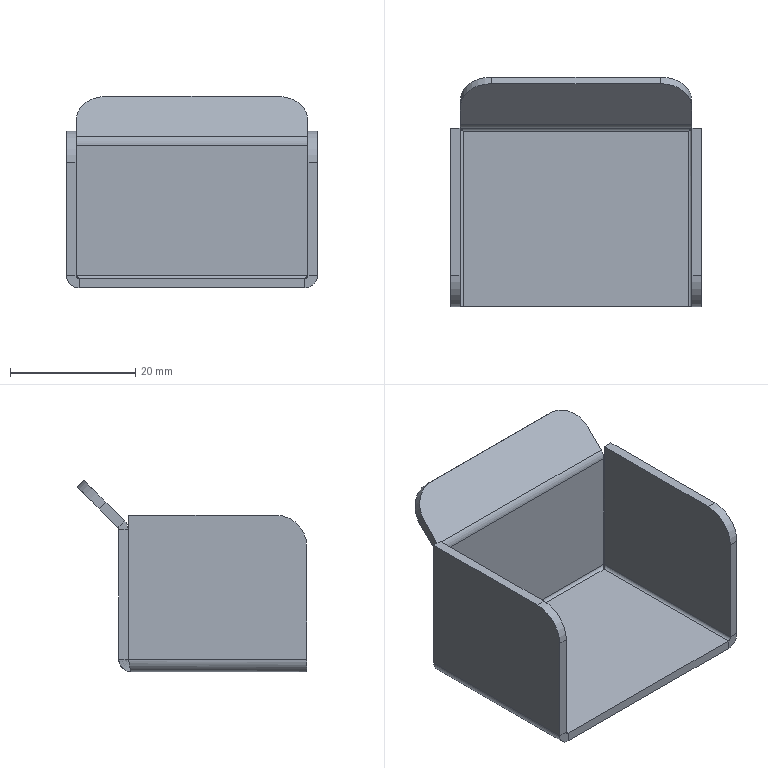Part | SolidWorks | features BaseBody 1 | 1 solid | 42 faces | box 40 x 36.632 x 30.571 mm | volume 5419 mm3 | plane 26 | cylinder 12 | spline 4 | commonest cylinder face diameters 1 x4 4 x4 10 x4
STEP:
#1=CARTESIAN_POINT('',(-13.429,20.571,29.071));
#2=VERTEX_POINT('',#1);
#3=CARTESIAN_POINT('',(-18.429,17.036,25.536));
#4=VERTEX_POINT('',#3);
#5=CARTESIAN_POINT('',(-13.429,17.036,25.536));
#6=DIRECTION('',(0.,-0.7071,0.7071));
#7=DIRECTION('',(0.,0.7071,0.7071));
#8=AXIS2_PLACEMENT_3D('',#5,#6,#7);
#9=CIRCLE('',#8,5.);
#10=EDGE_CURVE('',#2,#4,#9,.T.);
#11=ORIENTED_EDGE('',*,*,#10,.F.);
#12=CARTESIAN_POINT('',(-13.429,21.632,28.01));
#13=VERTEX_POINT('',#12);
#14=CARTESIAN_POINT('',(-13.429,20.571,29.071));
#15=DIRECTION('',(0.,-0.7071,0.7071));
#16=VECTOR('',#15,1000.);
#17=LINE('',#14,#16);
#18=EDGE_CURVE('',#13,#2,#17,.T.);
#19=ORIENTED_EDGE('',*,*,#18,.F.);
#20=CARTESIAN_POINT('',(-18.429,18.096,24.475));
#21=VERTEX_POINT('',#20);
#22=CARTESIAN_POINT('',(-13.429,18.096,24.475));
#23=DIRECTION('',(0.,0.7071,-0.7071));
#24=DIRECTION('',(0.,0.7071,0.7071));
#25=AXIS2_PLACEMENT_3D('',#22,#23,#24);
#26=CIRCLE('',#25,5.);
#27=EDGE_CURVE('',#21,#13,#26,.T.);
#28=ORIENTED_EDGE('',*,*,#27,.F.);
#29=CARTESIAN_POINT('',(-18.429,17.036,25.536));
#30=DIRECTION('',(0.,0.7071,-0.7071));
#31=VECTOR('',#30,1000.);
#32=LINE('',#29,#31);
#33=EDGE_CURVE('',#4,#21,#32,.T.);
#34=ORIENTED_EDGE('',*,*,#33,.F.);
#35=EDGE_LOOP('',(#11,#19,#28,#34));
#36=FACE_OUTER_BOUND('',#35,.T.);
#37=CARTESIAN_POINT('',(-13.429,17.036,25.536));
#38=DIRECTION('',(0.,0.7071,-0.7071));
#39=DIRECTION('',(0.,0.7071,0.7071));
#40=AXIS2_PLACEMENT_3D('',#37,#38,#39);
#41=CYLINDRICAL_SURFACE('',#40,5.);
#42=ADVANCED_FACE('',(#36),#41,.T.);
#43=CARTESIAN_POINT('',(18.429,17.036,25.536));
#44=VERTEX_POINT('',#43);
#45=CARTESIAN_POINT('',(13.429,20.571,29.071));
#46=VERTEX_POINT('',#45);
#47=CARTESIAN_POINT('',(13.429,17.036,25.536));
#48=DIRECTION('',(0.,-0.7071,0.7071));
#49=DIRECTION('',(0.,0.7071,0.7071));
#50=AXIS2_PLACEMENT_3D('',#47,#48,#49);
#51=CIRCLE('',#50,5.);
#52=EDGE_CURVE('',#44,#46,#51,.T.);
#53=ORIENTED_EDGE('',*,*,#52,.F.);
#54=CARTESIAN_POINT('',(18.429,18.096,24.475));
#55=VERTEX_POINT('',#54);
#56=CARTESIAN_POINT('',(18.429,17.036,25.536));
#57=DIRECTION('',(0.,-0.7071,0.7071));
#58=VECTOR('',#57,1000.);
#59=LINE('',#56,#58);
#60=EDGE_CURVE('',#55,#44,#59,.T.);
#61=ORIENTED_EDGE('',*,*,#60,.F.);
#62=CARTESIAN_POINT('',(13.429,21.632,28.01));
#63=VERTEX_POINT('',#62);
#64=CARTESIAN_POINT('',(13.429,18.096,24.475));
#65=DIRECTION('',(0.,0.7071,-0.7071));
#66=DIRECTION('',(0.,0.7071,0.7071));
#67=AXIS2_PLACEMENT_3D('',#64,#65,#66);
#68=CIRCLE('',#67,5.);
#69=EDGE_CURVE('',#63,#55,#68,.T.);
#70=ORIENTED_EDGE('',*,*,#69,.F.);
#71=CARTESIAN_POINT('',(13.429,20.571,29.071));
#72=DIRECTION('',(0.,0.7071,-0.7071));
#73=VECTOR('',#72,1000.);
#74=LINE('',#71,#73);
#75=EDGE_CURVE('',#46,#63,#74,.T.);
#76=ORIENTED_EDGE('',*,*,#75,.F.);
#77=EDGE_LOOP('',(#53,#61,#70,#76));
#78=FACE_OUTER_BOUND('',#77,.T.);
#79=CARTESIAN_POINT('',(13.429,17.036,25.536));
#80=DIRECTION('',(0.,0.7071,-0.7071));
#81=DIRECTION('',(0.,0.7071,0.7071));
#82=AXIS2_PLACEMENT_3D('',#79,#80,#81);
#83=CYLINDRICAL_SURFACE('',#82,5.);
#84=ADVANCED_FACE('',(#78),#83,.T.);
#85=CARTESIAN_POINT('',(20.,-10.,23.5));
#86=VERTEX_POINT('',#85);
#87=CARTESIAN_POINT('',(20.,-15.,18.5));
#88=VERTEX_POINT('',#87);
#89=CARTESIAN_POINT('',(20.,-10.,18.5));
#90=DIRECTION('',(1.,0.,0.));
#91=DIRECTION('',(0.,0.,1.));
#92=AXIS2_PLACEMENT_3D('',#89,#90,#91);
#93=CIRCLE('',#92,5.);
#94=EDGE_CURVE('',#86,#88,#93,.T.);
#95=ORIENTED_EDGE('',*,*,#94,.F.);
#96=CARTESIAN_POINT('',(18.5,-10.,23.5));
#97=VERTEX_POINT('',#96);
#98=CARTESIAN_POINT('',(20.,-10.,23.5));
#99=DIRECTION('',(1.,0.,0.));
#100=VECTOR('',#99,1000.);
#101=LINE('',#98,#100);
#102=EDGE_CURVE('',#97,#86,#101,.T.);
#103=ORIENTED_EDGE('',*,*,#102,.F.);
#104=CARTESIAN_POINT('',(18.5,-15.,18.5));
#105=VERTEX_POINT('',#104);
#106=CARTESIAN_POINT('',(18.5,-10.,18.5));
#107=DIRECTION('',(-1.,0.,0.));
#108=DIRECTION('',(0.,0.,1.));
#109=AXIS2_PLACEMENT_3D('',#106,#107,#108);
#110=CIRCLE('',#109,5.);
#111=EDGE_CURVE('',#105,#97,#110,.T.);
#112=ORIENTED_EDGE('',*,*,#111,.F.);
#113=CARTESIAN_POINT('',(20.,-15.,18.5));
#114=DIRECTION('',(-1.,0.,0.));
#115=VECTOR('',#114,1000.);
#116=LINE('',#113,#115);
#117=EDGE_CURVE('',#88,#105,#116,.T.);
#118=ORIENTED_EDGE('',*,*,#117,.F.);
#119=EDGE_LOOP('',(#95,#103,#112,#118));
#120=FACE_OUTER_BOUND('',#119,.T.);
#121=CARTESIAN_POINT('',(20.,-10.,18.5));
#122=DIRECTION('',(-1.,0.,0.));
#123=DIRECTION('',(0.,0.,1.));
#124=AXIS2_PLACEMENT_3D('',#121,#122,#123);
#125=CYLINDRICAL_SURFACE('',#124,5.);
#126=ADVANCED_FACE('',(#120),#125,.T.);
#127=CARTESIAN_POINT('',(-20.,-15.,18.5));
#128=VERTEX_POINT('',#127);
#129=CARTESIAN_POINT('',(-20.,-10.,23.5));
#130=VERTEX_POINT('',#129);
#131=CARTESIAN_POINT('',(-20.,-10.,18.5));
#132=DIRECTION('',(-1.,0.,0.));
#133=DIRECTION('',(0.,0.,-1.));
#134=AXIS2_PLACEMENT_3D('',#131,#132,#133);
#135=CIRCLE('',#134,5.);
#136=EDGE_CURVE('',#128,#130,#135,.T.);
#137=ORIENTED_EDGE('',*,*,#136,.F.);
#138=CARTESIAN_POINT('',(-18.5,-15.,18.5));
#139=VERTEX_POINT('',#138);
#140=CARTESIAN_POINT('',(-20.,-15.,18.5));
#141=DIRECTION('',(-1.,0.,0.));
#142=VECTOR('',#141,1000.);
#143=LINE('',#140,#142);
#144=EDGE_CURVE('',#139,#128,#143,.T.);
#145=ORIENTED_EDGE('',*,*,#144,.F.);
#146=CARTESIAN_POINT('',(-18.5,-10.,23.5));
#147=VERTEX_POINT('',#146);
#148=CARTESIAN_POINT('',(-18.5,-10.,18.5));
#149=DIRECTION('',(1.,0.,0.));
#150=DIRECTION('',(0.,0.,-1.));
#151=AXIS2_PLACEMENT_3D('',#148,#149,#150);
#152=CIRCLE('',#151,5.);
#153=EDGE_CURVE('',#147,#139,#152,.T.);
#154=ORIENTED_EDGE('',*,*,#153,.F.);
#155=CARTESIAN_POINT('',(-20.,-10.,23.5));
#156=DIRECTION('',(1.,0.,0.));
#157=VECTOR('',#156,1000.);
#158=LINE('',#155,#157);
#159=EDGE_CURVE('',#130,#147,#158,.T.);
#160=ORIENTED_EDGE('',*,*,#159,.F.);
#161=EDGE_LOOP('',(#137,#145,#154,#160));
#162=FACE_OUTER_BOUND('',#161,.T.);
#163=CARTESIAN_POINT('',(-20.,-10.,18.5));
#164=DIRECTION('',(1.,0.,0.));
#165=DIRECTION('',(0.,0.,-1.));
#166=AXIS2_PLACEMENT_3D('',#163,#164,#165);
#167=CYLINDRICAL_SURFACE('',#166,5.);
#168=ADVANCED_FACE('',(#162),#167,.T.);
#169=CARTESIAN_POINT('',(0.,20.571,29.071));
#170=DIRECTION('',(-1.,0.,0.));
#171=VECTOR('',#170,1000.);
#172=LINE('',#169,#171);
#173=EDGE_CURVE('',#46,#2,#172,.T.);
#174=ORIENTED_EDGE('',*,*,#173,.F.);
#175=ORIENTED_EDGE('',*,*,#75,.T.);
#176=CARTESIAN_POINT('',(-18.429,21.632,28.01));
#177=DIRECTION('',(-1.,0.,0.));
#178=VECTOR('',#177,1000.);
#179=LINE('',#176,#178);
#180=EDGE_CURVE('',#63,#13,#179,.T.);
#181=ORIENTED_EDGE('',*,*,#180,.T.);
#182=ORIENTED_EDGE('',*,*,#18,.T.);
#183=EDGE_LOOP('',(#174,#175,#181,#182));
#184=FACE_OUTER_BOUND('',#183,.T.);
#185=CARTESIAN_POINT('',(-18.429,20.571,29.071));
#186=DIRECTION('',(0.,-0.7071,-0.7071));
#187=DIRECTION('',(0.,-0.7071,0.7071));
#188=AXIS2_PLACEMENT_3D('',#185,#186,#187);
#189=PLANE('',#188);
#190=ADVANCED_FACE('',(#184),#189,.F.);
#191=ORIENTED_EDGE('',*,*,#180,.F.);
#192=ORIENTED_EDGE('',*,*,#69,.T.);
#193=CARTESIAN_POINT('',(18.429,15.146,21.525));
#194=VERTEX_POINT('',#193);
#195=CARTESIAN_POINT('',(18.429,21.632,28.01));
#196=DIRECTION('',(0.,0.7071,0.7071));
#197=VECTOR('',#196,1000.);
#198=LINE('',#195,#197);
#199=EDGE_CURVE('',#194,#55,#198,.T.);
#200=ORIENTED_EDGE('',*,*,#199,.F.);
#201=CARTESIAN_POINT('',(-18.429,15.146,21.525));
#202=VERTEX_POINT('',#201);
#203=CARTESIAN_POINT('',(-18.429,15.146,21.525));
#204=DIRECTION('',(1.,0.,0.));
#205=VECTOR('',#204,1000.);
#206=LINE('',#203,#205);
#207=EDGE_CURVE('',#202,#194,#206,.T.);
#208=ORIENTED_EDGE('',*,*,#207,.F.);
#209=CARTESIAN_POINT('',(-18.429,15.,21.379));
#210=DIRECTION('',(0.,-0.7071,-0.7071));
#211=VECTOR('',#210,1000.);
#212=LINE('',#209,#211);
#213=EDGE_CURVE('',#21,#202,#212,.T.);
#214=ORIENTED_EDGE('',*,*,#213,.F.);
#215=ORIENTED_EDGE('',*,*,#27,.T.);
#216=EDGE_LOOP('',(#191,#192,#200,#208,#214,#215));
#217=FACE_OUTER_BOUND('',#216,.T.);
#218=CARTESIAN_POINT('',(0.,-4.25,2.129));
#219=DIRECTION('',(0.,0.7071,-0.7071));
#220=DIRECTION('',(-1.,0.,0.));
#221=AXIS2_PLACEMENT_3D('',#218,#219,#220);
#222=PLANE('',#221);
#223=ADVANCED_FACE('',(#217),#222,.T.);
#224=CARTESIAN_POINT('',(18.429,14.086,22.586));
#225=VERTEX_POINT('',#224);
#226=CARTESIAN_POINT('',(18.429,-5.311,3.189));
#227=DIRECTION('',(0.,0.7071,0.7071));
#228=VECTOR('',#227,1000.);
#229=LINE('',#226,#228);
#230=EDGE_CURVE('',#225,#44,#229,.T.);
#231=ORIENTED_EDGE('',*,*,#230,.T.);
#232=ORIENTED_EDGE('',*,*,#52,.T.);
#233=ORIENTED_EDGE('',*,*,#173,.T.);
#234=ORIENTED_EDGE('',*,*,#10,.T.);
#235=CARTESIAN_POINT('',(-18.429,14.086,22.586));
#236=VERTEX_POINT('',#235);
#237=CARTESIAN_POINT('',(-18.429,-5.311,3.189));
#238=DIRECTION('',(0.,-0.7071,-0.7071));
#239=VECTOR('',#238,1000.);
#240=LINE('',#237,#239);
#241=EDGE_CURVE('',#4,#236,#240,.T.);
#242=ORIENTED_EDGE('',*,*,#241,.T.);
#243=CARTESIAN_POINT('',(-18.429,14.086,22.586));
#244=DIRECTION('',(-1.,0.,0.));
#245=VECTOR('',#244,1000.);
#246=LINE('',#243,#245);
#247=EDGE_CURVE('',#225,#236,#246,.T.);
#248=ORIENTED_EDGE('',*,*,#247,.F.);
#249=EDGE_LOOP('',(#231,#232,#233,#234,#242,#248));
#250=FACE_OUTER_BOUND('',#249,.T.);
#251=CARTESIAN_POINT('',(0.,-5.311,3.189));
#252=DIRECTION('',(0.,0.7071,-0.7071));
#253=DIRECTION('',(-1.,0.,0.));
#254=AXIS2_PLACEMENT_3D('',#251,#252,#253);
#255=PLANE('',#254);
#256=ADVANCED_FACE('',(#250),#255,.F.);
#257=ORIENTED_EDGE('',*,*,#199,.T.);
#258=ORIENTED_EDGE('',*,*,#60,.T.);
#259=ORIENTED_EDGE('',*,*,#230,.F.);
#260=CARTESIAN_POINT('',(18.429,15.146,21.525));
#261=DIRECTION('',(0.,-0.7071,0.7071));
#262=VECTOR('',#261,1000.);
#263=LINE('',#260,#262);
#264=EDGE_CURVE('',#194,#225,#263,.T.);
#265=ORIENTED_EDGE('',*,*,#264,.F.);
#266=EDGE_LOOP('',(#257,#258,#259,#265));
#267=FACE_OUTER_BOUND('',#266,.T.);
#268=CARTESIAN_POINT('',(18.429,20.571,29.071));
#269=DIRECTION('',(-1.,0.,0.));
#270=DIRECTION('',(0.,1.,0.));
#271=AXIS2_PLACEMENT_3D('',#268,#269,#270);
#272=PLANE('',#271);
#273=ADVANCED_FACE('',(#267),#272,.F.);
#274=ORIENTED_EDGE('',*,*,#241,.F.);
#275=ORIENTED_EDGE('',*,*,#33,.T.);
#276=ORIENTED_EDGE('',*,*,#213,.T.);
#277=CARTESIAN_POINT('',(-18.429,14.086,22.586));
#278=DIRECTION('',(0.,-0.7071,0.7071));
#279=VECTOR('',#278,1000.);
#280=LINE('',#277,#279);
#281=EDGE_CURVE('',#202,#236,#280,.T.);
#282=ORIENTED_EDGE('',*,*,#281,.T.);
#283=EDGE_LOOP('',(#274,#275,#276,#282));
#284=FACE_OUTER_BOUND('',#283,.T.);
#285=CARTESIAN_POINT('',(-18.429,13.939,22.439));
#286=DIRECTION('',(1.,0.,0.));
#287=DIRECTION('',(0.,1.,0.));
#288=AXIS2_PLACEMENT_3D('',#285,#286,#287);
#289=PLANE('',#288);
#290=ADVANCED_FACE('',(#284),#289,.F.);
#291=CARTESIAN_POINT('',(18.429,15.,21.172));
#292=VERTEX_POINT('',#291);
#293=CARTESIAN_POINT('',(-18.429,15.,21.172));
#294=VERTEX_POINT('',#293);
#295=CARTESIAN_POINT('',(18.429,15.,21.172));
#296=DIRECTION('',(-1.,0.,0.));
#297=VECTOR('',#296,1000.);
#298=LINE('',#295,#297);
#299=EDGE_CURVE('',#292,#294,#298,.T.);
#300=ORIENTED_EDGE('',*,*,#299,.T.);
#301=CARTESIAN_POINT('',(-18.429,15.5,21.172));
#302=DIRECTION('',(-1.,0.,0.));
#303=DIRECTION('',(0.,0.,-1.));
#304=AXIS2_PLACEMENT_3D('',#301,#302,#303);
#305=CIRCLE('',#304,0.5);
#306=EDGE_CURVE('',#294,#202,#305,.T.);
#307=ORIENTED_EDGE('',*,*,#306,.T.);
#308=ORIENTED_EDGE('',*,*,#207,.T.);
#309=CARTESIAN_POINT('',(18.429,15.5,21.172));
#310=DIRECTION('',(1.,0.,0.));
#311=DIRECTION('',(0.,0.,-1.));
#312=AXIS2_PLACEMENT_3D('',#309,#310,#311);
#313=CIRCLE('',#312,0.5);
#314=EDGE_CURVE('',#194,#292,#313,.T.);
#315=ORIENTED_EDGE('',*,*,#314,.T.);
#316=EDGE_LOOP('',(#300,#307,#308,#315));
#317=FACE_OUTER_BOUND('',#316,.T.);
#318=CARTESIAN_POINT('',(18.429,15.5,21.172));
#319=DIRECTION('',(1.,0.,0.));
#320=DIRECTION('',(0.,-0.7071,0.7071));
#321=AXIS2_PLACEMENT_3D('',#318,#319,#320);
#322=CYLINDRICAL_SURFACE('',#321,0.5);
#323=ADVANCED_FACE('',(#317),#322,.F.);
#324=CARTESIAN_POINT('',(18.429,13.5,21.172));
#325=VERTEX_POINT('',#324);
#326=CARTESIAN_POINT('',(-18.429,13.5,21.172));
#327=VERTEX_POINT('',#326);
#328=CARTESIAN_POINT('',(18.429,13.5,21.172));
#329=DIRECTION('',(-1.,0.,0.));
#330=VECTOR('',#329,1000.);
#331=LINE('',#328,#330);
#332=EDGE_CURVE('',#325,#327,#331,.T.);
#333=ORIENTED_EDGE('',*,*,#332,.F.);
#334=CARTESIAN_POINT('',(18.429,15.5,21.172));
#335=DIRECTION('',(1.,0.,0.));
#336=DIRECTION('',(0.,0.,-1.));
#337=AXIS2_PLACEMENT_3D('',#334,#335,#336);
#338=CIRCLE('',#337,2.);
#339=EDGE_CURVE('',#225,#325,#338,.T.);
#340=ORIENTED_EDGE('',*,*,#339,.F.);
#341=ORIENTED_EDGE('',*,*,#247,.T.);
#342=CARTESIAN_POINT('',(-18.429,15.5,21.172));
#343=DIRECTION('',(-1.,0.,0.));
#344=DIRECTION('',(0.,0.,-1.));
#345=AXIS2_PLACEMENT_3D('',#342,#343,#344);
#346=CIRCLE('',#345,2.);
#347=EDGE_CURVE('',#327,#236,#346,.T.);
#348=ORIENTED_EDGE('',*,*,#347,.F.);
#349=EDGE_LOOP('',(#333,#340,#341,#348));
#350=FACE_OUTER_BOUND('',#349,.T.);
#351=CARTESIAN_POINT('',(18.429,15.5,21.172));
#352=DIRECTION('',(1.,0.,0.));
#353=DIRECTION('',(0.,-0.7071,0.7071));
#354=AXIS2_PLACEMENT_3D('',#351,#352,#353);
#355=CYLINDRICAL_SURFACE('',#354,2.);
#356=ADVANCED_FACE('',(#350),#355,.T.);
#357=ORIENTED_EDGE('',*,*,#314,.F.);
#358=ORIENTED_EDGE('',*,*,#264,.T.);
#359=ORIENTED_EDGE('',*,*,#339,.T.);
#360=CARTESIAN_POINT('',(18.429,15.,21.172));
#361=DIRECTION('',(0.,-1.,0.));
#362=VECTOR('',#361,1000.);
#363=LINE('',#360,#362);
#364=EDGE_CURVE('',#292,#325,#363,.T.);
#365=ORIENTED_EDGE('',*,*,#364,.F.);
#366=EDGE_LOOP('',(#357,#358,#359,#365));
#367=FACE_OUTER_BOUND('',#366,.T.);
#368=CARTESIAN_POINT('',(18.429,15.5,21.172));
#369=DIRECTION('',(-1.,0.,0.));
#370=DIRECTION('',(0.,0.,1.));
#371=AXIS2_PLACEMENT_3D('',#368,#369,#370);
#372=PLANE('',#371);
#373=ADVANCED_FACE('',(#367),#372,.F.);
#374=ORIENTED_EDGE('',*,*,#281,.F.);
#375=ORIENTED_EDGE('',*,*,#306,.F.);
#376=CARTESIAN_POINT('',(-18.429,15.,21.172));
#377=DIRECTION('',(0.,-1.,0.));
#378=VECTOR('',#377,1000.);
#379=LINE('',#376,#378);
#380=EDGE_CURVE('',#294,#327,#379,.T.);
#381=ORIENTED_EDGE('',*,*,#380,.T.);
#382=ORIENTED_EDGE('',*,*,#347,.T.);
#383=EDGE_LOOP('',(#374,#375,#381,#382));
#384=FACE_OUTER_BOUND('',#383,.T.);
#385=CARTESIAN_POINT('',(-18.429,15.5,21.172));
#386=DIRECTION('',(-1.,0.,0.));
#387=DIRECTION('',(0.,0.,1.));
#388=AXIS2_PLACEMENT_3D('',#385,#386,#387);
#389=PLANE('',#388);
#390=ADVANCED_FACE('',(#384),#389,.T.);
#391=CARTESIAN_POINT('',(20.,13.429,23.5));
#392=VERTEX_POINT('',#391);
#393=CARTESIAN_POINT('',(18.5,13.429,23.5));
#394=VERTEX_POINT('',#393);
#395=CARTESIAN_POINT('',(20.,13.429,23.5));
#396=DIRECTION('',(-1.,0.,0.));
#397=VECTOR('',#396,1000.);
#398=LINE('',#395,#397);
#399=EDGE_CURVE('',#392,#394,#398,.T.);
#400=ORIENTED_EDGE('',*,*,#399,.F.);
#401=CARTESIAN_POINT('',(20.,13.429,0.5));
#402=VERTEX_POINT('',#401);
#403=CARTESIAN_POINT('',(20.,13.429,0.));
#404=DIRECTION('',(0.,0.,1.));
#405=VECTOR('',#404,1000.);
#406=LINE('',#403,#405);
#407=EDGE_CURVE('',#402,#392,#406,.T.);
#408=ORIENTED_EDGE('',*,*,#407,.F.);
#409=CARTESIAN_POINT('',(18.5,13.429,0.5));
#410=VERTEX_POINT('',#409);
#411=CARTESIAN_POINT('',(18.5,13.429,0.5));
#412=DIRECTION('',(-1.,0.,0.));
#413=VECTOR('',#412,1000.);
#414=LINE('',#411,#413);
#415=EDGE_CURVE('',#402,#410,#414,.T.);
#416=ORIENTED_EDGE('',*,*,#415,.T.);
#417=CARTESIAN_POINT('',(18.5,13.429,0.));
#418=DIRECTION('',(0.,0.,1.));
#419=VECTOR('',#418,1000.);
#420=LINE('',#417,#419);
#421=EDGE_CURVE('',#410,#394,#420,.T.);
#422=ORIENTED_EDGE('',*,*,#421,.T.);
#423=EDGE_LOOP('',(#400,#408,#416,#422));
#424=FACE_OUTER_BOUND('',#423,.T.);
#425=CARTESIAN_POINT('',(18.5,13.429,0.));
#426=DIRECTION('',(0.,-1.,0.));
#427=DIRECTION('',(0.,0.,-1.));
#428=AXIS2_PLACEMENT_3D('',#425,#426,#427);
#429=PLANE('',#428);
#430=ADVANCED_FACE('',(#424),#429,.F.);
#431=CARTESIAN_POINT('',(18.5,-15.,23.5));
#432=DIRECTION('',(0.,-1.,0.));
#433=VECTOR('',#432,1000.);
#434=LINE('',#431,#433);
#435=EDGE_CURVE('',#394,#97,#434,.T.);
#436=ORIENTED_EDGE('',*,*,#435,.T.);
#437=ORIENTED_EDGE('',*,*,#102,.T.);
#438=CARTESIAN_POINT('',(20.,0.,23.5));
#439=DIRECTION('',(0.,-1.,0.));
#440=VECTOR('',#439,1000.);
#441=LINE('',#438,#440);
#442=EDGE_CURVE('',#392,#86,#441,.T.);
#443=ORIENTED_EDGE('',*,*,#442,.F.);
#444=ORIENTED_EDGE('',*,*,#399,.T.);
#445=EDGE_LOOP('',(#436,#437,#443,#444));
#446=FACE_OUTER_BOUND('',#445,.T.);
#447=CARTESIAN_POINT('',(20.,-15.,23.5));
#448=DIRECTION('',(0.,0.,-1.));
#449=DIRECTION('',(-1.,0.,0.));
#450=AXIS2_PLACEMENT_3D('',#447,#448,#449);
#451=PLANE('',#450);
#452=ADVANCED_FACE('',(#446),#451,.F.);
#453=CARTESIAN_POINT('',(18.5,-15.,0.5));
#454=VERTEX_POINT('',#453);
#455=CARTESIAN_POINT('',(18.5,-15.,0.));
#456=DIRECTION('',(0.,0.,-1.));
#457=VECTOR('',#456,1000.);
#458=LINE('',#455,#457);
#459=EDGE_CURVE('',#105,#454,#458,.T.);
#460=ORIENTED_EDGE('',*,*,#459,.F.);
#461=ORIENTED_EDGE('',*,*,#111,.T.);
#462=ORIENTED_EDGE('',*,*,#435,.F.);
#463=ORIENTED_EDGE('',*,*,#421,.F.);
#464=CARTESIAN_POINT('',(18.5,-15.,0.5));
#465=DIRECTION('',(0.,1.,0.));
#466=VECTOR('',#465,1000.);
#467=LINE('',#464,#466);
#468=EDGE_CURVE('',#454,#410,#467,.T.);
#469=ORIENTED_EDGE('',*,*,#468,.F.);
#470=EDGE_LOOP('',(#460,#461,#462,#463,#469));
#471=FACE_OUTER_BOUND('',#470,.T.);
#472=CARTESIAN_POINT('',(18.5,0.,0.));
#473=DIRECTION('',(-1.,0.,0.));
#474=DIRECTION('',(0.,1.,0.));
#475=AXIS2_PLACEMENT_3D('',#472,#473,#474);
#476=PLANE('',#475);
#477=ADVANCED_FACE('',(#471),#476,.T.);
#478=ORIENTED_EDGE('',*,*,#442,.T.);
#479=ORIENTED_EDGE('',*,*,#94,.T.);
#480=CARTESIAN_POINT('',(20.,-15.,0.5));
#481=VERTEX_POINT('',#480);
#482=CARTESIAN_POINT('',(20.,-15.,0.));
#483=DIRECTION('',(0.,0.,-1.));
#484=VECTOR('',#483,1000.);
#485=LINE('',#482,#484);
#486=EDGE_CURVE('',#88,#481,#485,.T.);
#487=ORIENTED_EDGE('',*,*,#486,.T.);
#488=CARTESIAN_POINT('',(20.,-15.,0.5));
#489=DIRECTION('',(0.,-1.,0.));
#490=VECTOR('',#489,1000.);
#491=LINE('',#488,#490);
#492=EDGE_CURVE('',#402,#481,#491,.T.);
#493=ORIENTED_EDGE('',*,*,#492,.F.);
#494=ORIENTED_EDGE('',*,*,#407,.T.);
#495=EDGE_LOOP('',(#478,#479,#487,#493,#494));
#496=FACE_OUTER_BOUND('',#495,.T.);
#497=CARTESIAN_POINT('',(20.,0.,0.));
#498=DIRECTION('',(-1.,0.,0.));
#499=DIRECTION('',(0.,1.,0.));
#500=AXIS2_PLACEMENT_3D('',#497,#498,#499);
#501=PLANE('',#500);
#502=ADVANCED_FACE('',(#496),#501,.F.);
#503=ORIENTED_EDGE('',*,*,#486,.F.);
#504=ORIENTED_EDGE('',*,*,#117,.T.);
#505=ORIENTED_EDGE('',*,*,#459,.T.);
#506=CARTESIAN_POINT('',(20.,-15.,0.5));
#507=DIRECTION('',(1.,0.,0.));
#508=VECTOR('',#507,1000.);
#509=LINE('',#506,#508);
#510=EDGE_CURVE('',#454,#481,#509,.T.);
#511=ORIENTED_EDGE('',*,*,#510,.T.);
#512=EDGE_LOOP('',(#503,#504,#505,#511));
#513=FACE_OUTER_BOUND('',#512,.T.);
#514=CARTESIAN_POINT('',(20.,-15.,0.));
#515=DIRECTION('',(0.,1.,0.));
#516=DIRECTION('',(0.,0.,-1.));
#517=AXIS2_PLACEMENT_3D('',#514,#515,#516);
#518=PLANE('',#517);
#519=ADVANCED_FACE('',(#513),#518,.F.);
#520=CARTESIAN_POINT('',(18.,13.,0.));
#521=VERTEX_POINT('',#520);
#522=CARTESIAN_POINT('',(18.,-15.,0.));
#523=VERTEX_POINT('',#522);
#524=CARTESIAN_POINT('',(18.,13.429,0.));
#525=DIRECTION('',(0.,-1.,0.));
#526=VECTOR('',#525,1000.);
#527=LINE('',#524,#526);
#528=EDGE_CURVE('',#521,#523,#527,.T.);
#529=ORIENTED_EDGE('',*,*,#528,.T.);
#530=CARTESIAN_POINT('',(18.,-15.,0.5));
#531=DIRECTION('',(0.,-1.,0.));
#532=DIRECTION('',(0.,0.,1.));
#533=AXIS2_PLACEMENT_3D('',#530,#531,#532);
#534=CIRCLE('',#533,0.5);
#535=EDGE_CURVE('',#523,#454,#534,.T.);
#536=ORIENTED_EDGE('',*,*,#535,.T.);
#537=ORIENTED_EDGE('',*,*,#468,.T.);
#538=CARTESIAN_POINT('',(18.5,13.429,0.5));
#539=CARTESIAN_POINT('',(18.5,13.358,0.3691));
#540=CARTESIAN_POINT('',(18.446,13.286,0.239));
#541=CARTESIAN_POINT('',(18.261,13.143,0.05389));
#542=CARTESIAN_POINT('',(18.131,13.072,0.));
#543=CARTESIAN_POINT('',(18.,13.,0.));
#544=B_SPLINE_CURVE_WITH_KNOTS('',3,(#538,#539,#540,#541,#542,#543),.UNSPECIFIED.,.F.,.F.,(4,2,4),(0.,0.5,1.),.UNSPECIFIED.);
#545=EDGE_CURVE('',#410,#521,#544,.T.);
#546=ORIENTED_EDGE('',*,*,#545,.T.);
#547=EDGE_LOOP('',(#529,#536,#537,#546));
#548=FACE_OUTER_BOUND('',#547,.T.);
#549=CARTESIAN_POINT('',(18.,13.429,0.5));
#550=DIRECTION('',(0.,1.,0.));
#551=DIRECTION('',(1.,0.,0.));
#552=AXIS2_PLACEMENT_3D('',#549,#550,#551);
#553=CYLINDRICAL_SURFACE('',#552,0.5);
#554=ADVANCED_FACE('',(#548),#553,.F.);
#555=CARTESIAN_POINT('',(18.,13.,-1.5));
#556=VERTEX_POINT('',#555);
#557=CARTESIAN_POINT('',(18.,-15.,-1.5));
#558=VERTEX_POINT('',#557);
#559=CARTESIAN_POINT('',(18.,13.429,-1.5));
#560=DIRECTION('',(0.,-1.,0.));
#561=VECTOR('',#560,1000.);
#562=LINE('',#559,#561);
#563=EDGE_CURVE('',#556,#558,#562,.T.);
#564=ORIENTED_EDGE('',*,*,#563,.F.);
#565=CARTESIAN_POINT('',(20.,13.429,0.5));
#566=CARTESIAN_POINT('',(20.,13.394,0.2382));
#567=CARTESIAN_POINT('',(19.948,13.358,-0.0235));
#568=CARTESIAN_POINT('',(19.748,13.286,-0.5072));
#569=CARTESIAN_POINT('',(19.599,13.25,-0.7291));
#570=CARTESIAN_POINT('',(19.229,13.179,-1.099));
#571=CARTESIAN_POINT('',(19.007,13.143,-1.248));
#572=CARTESIAN_POINT('',(18.523,13.072,-1.448));
#573=CARTESIAN_POINT('',(18.262,13.036,-1.5));
#574=CARTESIAN_POINT('',(18.,13.,-1.5));
#575=B_SPLINE_CURVE_WITH_KNOTS('',3,(#565,#566,#567,#568,#569,#570,#571,#572,#573,#574),.UNSPECIFIED.,.F.,.F.,(4,2,2,2,4),(0.,0.25,0.5,0.75,1.),.UNSPECIFIED.);
#576=EDGE_CURVE('',#402,#556,#575,.T.);
#577=ORIENTED_EDGE('',*,*,#576,.F.);
#578=ORIENTED_EDGE('',*,*,#492,.T.);
#579=CARTESIAN_POINT('',(18.,-15.,0.5));
#580=DIRECTION('',(0.,-1.,0.));
#581=DIRECTION('',(0.,0.,1.));
#582=AXIS2_PLACEMENT_3D('',#579,#580,#581);
#583=CIRCLE('',#582,2.);
#584=EDGE_CURVE('',#558,#481,#583,.T.);
#585=ORIENTED_EDGE('',*,*,#584,.F.);
#586=EDGE_LOOP('',(#564,#577,#578,#585));
#587=FACE_OUTER_BOUND('',#586,.T.);
#588=CARTESIAN_POINT('',(18.,13.429,0.5));
#589=DIRECTION('',(0.,1.,0.));
#590=DIRECTION('',(1.,0.,0.));
#591=AXIS2_PLACEMENT_3D('',#588,#589,#590);
#592=CYLINDRICAL_SURFACE('',#591,2.);
#593=ADVANCED_FACE('',(#587),#592,.T.);
#594=ORIENTED_EDGE('',*,*,#545,.F.);
#595=ORIENTED_EDGE('',*,*,#415,.F.);
#596=ORIENTED_EDGE('',*,*,#576,.T.);
#597=CARTESIAN_POINT('',(18.,13.,0.));
#598=DIRECTION('',(0.,0.,-1.));
#599=VECTOR('',#598,1000.);
#600=LINE('',#597,#599);
#601=EDGE_CURVE('',#521,#556,#600,.T.);
#602=ORIENTED_EDGE('',*,*,#601,.F.);
#603=EDGE_LOOP('',(#594,#595,#596,#602));
#604=FACE_OUTER_BOUND('',#603,.T.);
#605=CARTESIAN_POINT('',(20.015,13.429,0.5));
#606=CARTESIAN_POINT('',(20.015,13.394,0.2362));
#607=CARTESIAN_POINT('',(19.963,13.358,-0.02742));
#608=CARTESIAN_POINT('',(19.761,13.286,-0.5148));
#609=CARTESIAN_POINT('',(19.611,13.25,-0.7383));
#610=CARTESIAN_POINT('',(19.238,13.179,-1.111));
#611=CARTESIAN_POINT('',(19.015,13.143,-1.261));
#612=CARTESIAN_POINT('',(18.527,13.072,-1.463));
#613=CARTESIAN_POINT('',(18.264,13.036,-1.515));
#614=CARTESIAN_POINT('',(18.,13.,-1.515));
#615=CARTESIAN_POINT('',(20.,13.429,0.5));
#616=CARTESIAN_POINT('',(20.,13.394,0.2382));
#617=CARTESIAN_POINT('',(19.948,13.358,-0.0235));
#618=CARTESIAN_POINT('',(19.748,13.286,-0.5072));
#619=CARTESIAN_POINT('',(19.599,13.25,-0.7291));
#620=CARTESIAN_POINT('',(19.229,13.179,-1.099));
#621=CARTESIAN_POINT('',(19.007,13.143,-1.248));
#622=CARTESIAN_POINT('',(18.523,13.072,-1.448));
#623=CARTESIAN_POINT('',(18.262,13.036,-1.5));
#624=CARTESIAN_POINT('',(18.,13.,-1.5));
#625=CARTESIAN_POINT('',(18.5,13.429,0.5));
#626=CARTESIAN_POINT('',(18.5,13.394,0.4345));
#627=CARTESIAN_POINT('',(18.487,13.358,0.3691));
#628=CARTESIAN_POINT('',(18.437,13.286,0.2482));
#629=CARTESIAN_POINT('',(18.4,13.25,0.1927));
#630=CARTESIAN_POINT('',(18.307,13.179,0.1002));
#631=CARTESIAN_POINT('',(18.252,13.143,0.06311));
#632=CARTESIAN_POINT('',(18.131,13.072,0.01301));
#633=CARTESIAN_POINT('',(18.065,13.036,0.));
#634=CARTESIAN_POINT('',(18.,13.,0.));
#635=CARTESIAN_POINT('',(18.485,13.429,0.5));
#636=CARTESIAN_POINT('',(18.485,13.394,0.4365));
#637=CARTESIAN_POINT('',(18.472,13.358,0.3731));
#638=CARTESIAN_POINT('',(18.424,13.286,0.2558));
#639=CARTESIAN_POINT('',(18.388,13.25,0.202));
#640=CARTESIAN_POINT('',(18.298,13.179,0.1123));
#641=CARTESIAN_POINT('',(18.244,13.143,0.07634));
#642=CARTESIAN_POINT('',(18.127,13.072,0.02777));
#643=CARTESIAN_POINT('',(18.063,13.036,0.01515));
#644=CARTESIAN_POINT('',(18.,13.,0.01515));
#645=B_SPLINE_SURFACE_WITH_KNOTS('',1,3,((#605,#606,#607,#608,#609,#610,#611,#612,#613,#614),(#615,#616,#617,#618,#619,#620,#621,#622,#623,#624),(#625,#626,#627,#628,#629,#630,#631,#632,#633,#634),(#635,#636,#637,#638,#639,#640,#641,#642,#643,#644)),.UNSPECIFIED.,.F.,.F.,.F.,(2,1,1,2),(4,2,2,2,4),(-0.01,0.,1.,1.01),(0.,0.25,0.5,0.75,1.),.UNSPECIFIED.);
#646=ADVANCED_FACE('',(#604),#645,.F.);
#647=ORIENTED_EDGE('',*,*,#510,.F.);
#648=ORIENTED_EDGE('',*,*,#535,.F.);
#649=CARTESIAN_POINT('',(18.,-15.,0.));
#650=DIRECTION('',(0.,0.,-1.));
#651=VECTOR('',#650,1000.);
#652=LINE('',#649,#651);
#653=EDGE_CURVE('',#523,#558,#652,.T.);
#654=ORIENTED_EDGE('',*,*,#653,.T.);
#655=ORIENTED_EDGE('',*,*,#584,.T.);
#656=EDGE_LOOP('',(#647,#648,#654,#655));
#657=FACE_OUTER_BOUND('',#656,.T.);
#658=CARTESIAN_POINT('',(18.,-15.,0.5));
#659=DIRECTION('',(0.,-1.,0.));
#660=DIRECTION('',(-1.,0.,0.));
#661=AXIS2_PLACEMENT_3D('',#658,#659,#660);
#662=PLANE('',#661);
#663=ADVANCED_FACE('',(#657),#662,.T.);
#664=CARTESIAN_POINT('',(-18.,13.,0.));
#665=VERTEX_POINT('',#664);
#666=CARTESIAN_POINT('',(-18.429,13.,0.));
#667=DIRECTION('',(1.,0.,0.));
#668=VECTOR('',#667,1000.);
#669=LINE('',#666,#668);
#670=EDGE_CURVE('',#665,#521,#669,.T.);
#671=ORIENTED_EDGE('',*,*,#670,.T.);
#672=CARTESIAN_POINT('',(18.429,13.5,0.5));
#673=VERTEX_POINT('',#672);
#674=CARTESIAN_POINT('',(18.,13.,0.));
#675=CARTESIAN_POINT('',(18.072,13.131,0.));
#676=CARTESIAN_POINT('',(18.143,13.261,0.05389));
#677=CARTESIAN_POINT('',(18.286,13.446,0.239));
#678=CARTESIAN_POINT('',(18.358,13.5,0.3691));
#679=CARTESIAN_POINT('',(18.429,13.5,0.5));
#680=B_SPLINE_CURVE_WITH_KNOTS('',3,(#674,#675,#676,#677,#678,#679),.UNSPECIFIED.,.F.,.F.,(4,2,4),(0.,0.5,1.),.UNSPECIFIED.);
#681=EDGE_CURVE('',#521,#673,#680,.T.);
#682=ORIENTED_EDGE('',*,*,#681,.T.);
#683=CARTESIAN_POINT('',(-18.429,13.5,0.5));
#684=VERTEX_POINT('',#683);
#685=CARTESIAN_POINT('',(20.,13.5,0.5));
#686=DIRECTION('',(-1.,0.,0.));
#687=VECTOR('',#686,1000.);
#688=LINE('',#685,#687);
#689=EDGE_CURVE('',#673,#684,#688,.T.);
#690=ORIENTED_EDGE('',*,*,#689,.T.);
#691=CARTESIAN_POINT('',(-18.429,13.5,0.5));
#692=CARTESIAN_POINT('',(-18.358,13.5,0.3691));
#693=CARTESIAN_POINT('',(-18.286,13.446,0.239));
#694=CARTESIAN_POINT('',(-18.143,13.261,0.05389));
#695=CARTESIAN_POINT('',(-18.072,13.131,0.));
#696=CARTESIAN_POINT('',(-18.,13.,0.));
#697=B_SPLINE_CURVE_WITH_KNOTS('',3,(#691,#692,#693,#694,#695,#696),.UNSPECIFIED.,.F.,.F.,(4,2,4),(0.,0.5,1.),.UNSPECIFIED.);
#698=EDGE_CURVE('',#684,#665,#697,.T.);
#699=ORIENTED_EDGE('',*,*,#698,.T.);
#700=EDGE_LOOP('',(#671,#682,#690,#699));
#701=FACE_OUTER_BOUND('',#700,.T.);
#702=CARTESIAN_POINT('',(-18.429,13.,0.5));
#703=DIRECTION('',(-1.,0.,0.));
#704=DIRECTION('',(0.,1.,0.));
#705=AXIS2_PLACEMENT_3D('',#702,#703,#704);
#706=CYLINDRICAL_SURFACE('',#705,0.5);
#707=ADVANCED_FACE('',(#701),#706,.F.);
#708=CARTESIAN_POINT('',(-18.,13.,-1.5));
#709=VERTEX_POINT('',#708);
#710=CARTESIAN_POINT('',(-18.429,13.,-1.5));
#711=DIRECTION('',(1.,0.,0.));
#712=VECTOR('',#711,1000.);
#713=LINE('',#710,#712);
#714=EDGE_CURVE('',#709,#556,#713,.T.);
#715=ORIENTED_EDGE('',*,*,#714,.F.);
#716=CARTESIAN_POINT('',(-18.429,15.,0.5));
#717=VERTEX_POINT('',#716);
#718=CARTESIAN_POINT('',(-18.429,15.,0.5));
#719=CARTESIAN_POINT('',(-18.394,15.,0.2382));
#720=CARTESIAN_POINT('',(-18.358,14.948,-0.0235));
#721=CARTESIAN_POINT('',(-18.286,14.748,-0.5072));
#722=CARTESIAN_POINT('',(-18.25,14.599,-0.7291));
#723=CARTESIAN_POINT('',(-18.179,14.229,-1.099));
#724=CARTESIAN_POINT('',(-18.143,14.007,-1.248));
#725=CARTESIAN_POINT('',(-18.072,13.523,-1.448));
#726=CARTESIAN_POINT('',(-18.036,13.262,-1.5));
#727=CARTESIAN_POINT('',(-18.,13.,-1.5));
#728=B_SPLINE_CURVE_WITH_KNOTS('',3,(#718,#719,#720,#721,#722,#723,#724,#725,#726,#727),.UNSPECIFIED.,.F.,.F.,(4,2,2,2,4),(0.,0.25,0.5,0.75,1.),.UNSPECIFIED.);
#729=EDGE_CURVE('',#717,#709,#728,.T.);
#730=ORIENTED_EDGE('',*,*,#729,.F.);
#731=CARTESIAN_POINT('',(18.429,15.,0.5));
#732=VERTEX_POINT('',#731);
#733=CARTESIAN_POINT('',(20.,15.,0.5));
#734=DIRECTION('',(1.,0.,0.));
#735=VECTOR('',#734,1000.);
#736=LINE('',#733,#735);
#737=EDGE_CURVE('',#717,#732,#736,.T.);
#738=ORIENTED_EDGE('',*,*,#737,.T.);
#739=CARTESIAN_POINT('',(18.,13.,-1.5));
#740=CARTESIAN_POINT('',(18.036,13.262,-1.5));
#741=CARTESIAN_POINT('',(18.072,13.523,-1.448));
#742=CARTESIAN_POINT('',(18.143,14.007,-1.248));
#743=CARTESIAN_POINT('',(18.179,14.229,-1.099));
#744=CARTESIAN_POINT('',(18.25,14.599,-0.7291));
#745=CARTESIAN_POINT('',(18.286,14.748,-0.5072));
#746=CARTESIAN_POINT('',(18.358,14.948,-0.0235));
#747=CARTESIAN_POINT('',(18.394,15.,0.2382));
#748=CARTESIAN_POINT('',(18.429,15.,0.5));
#749=B_SPLINE_CURVE_WITH_KNOTS('',3,(#739,#740,#741,#742,#743,#744,#745,#746,#747,#748),.UNSPECIFIED.,.F.,.F.,(4,2,2,2,4),(0.,0.25,0.5,0.75,1.),.UNSPECIFIED.);
#750=EDGE_CURVE('',#556,#732,#749,.T.);
#751=ORIENTED_EDGE('',*,*,#750,.F.);
#752=EDGE_LOOP('',(#715,#730,#738,#751));
#753=FACE_OUTER_BOUND('',#752,.T.);
#754=CARTESIAN_POINT('',(-18.429,13.,0.5));
#755=DIRECTION('',(-1.,0.,0.));
#756=DIRECTION('',(0.,1.,0.));
#757=AXIS2_PLACEMENT_3D('',#754,#755,#756);
#758=CYLINDRICAL_SURFACE('',#757,2.);
#759=ADVANCED_FACE('',(#753),#758,.T.);
#760=ORIENTED_EDGE('',*,*,#698,.F.);
#761=CARTESIAN_POINT('',(-18.429,13.5,0.5));
#762=DIRECTION('',(0.,-1.,0.));
#763=VECTOR('',#762,1000.);
#764=LINE('',#761,#763);
#765=EDGE_CURVE('',#717,#684,#764,.T.);
#766=ORIENTED_EDGE('',*,*,#765,.F.);
#767=ORIENTED_EDGE('',*,*,#729,.T.);
#768=CARTESIAN_POINT('',(-18.,13.,0.));
#769=DIRECTION('',(0.,0.,-1.));
#770=VECTOR('',#769,1000.);
#771=LINE('',#768,#770);
#772=EDGE_CURVE('',#665,#709,#771,.T.);
#773=ORIENTED_EDGE('',*,*,#772,.F.);
#774=EDGE_LOOP('',(#760,#766,#767,#773));
#775=FACE_OUTER_BOUND('',#774,.T.);
#776=CARTESIAN_POINT('',(-18.429,15.015,0.5));
#777=CARTESIAN_POINT('',(-18.394,15.015,0.2362));
#778=CARTESIAN_POINT('',(-18.358,14.963,-0.02742));
#779=CARTESIAN_POINT('',(-18.286,14.761,-0.5148));
#780=CARTESIAN_POINT('',(-18.25,14.611,-0.7383));
#781=CARTESIAN_POINT('',(-18.179,14.238,-1.111));
#782=CARTESIAN_POINT('',(-18.143,14.015,-1.261));
#783=CARTESIAN_POINT('',(-18.072,13.527,-1.463));
#784=CARTESIAN_POINT('',(-18.036,13.264,-1.515));
#785=CARTESIAN_POINT('',(-18.,13.,-1.515));
#786=CARTESIAN_POINT('',(-18.429,15.,0.5));
#787=CARTESIAN_POINT('',(-18.394,15.,0.2382));
#788=CARTESIAN_POINT('',(-18.358,14.948,-0.0235));
#789=CARTESIAN_POINT('',(-18.286,14.748,-0.5072));
#790=CARTESIAN_POINT('',(-18.25,14.599,-0.7291));
#791=CARTESIAN_POINT('',(-18.179,14.229,-1.099));
#792=CARTESIAN_POINT('',(-18.143,14.007,-1.248));
#793=CARTESIAN_POINT('',(-18.072,13.523,-1.448));
#794=CARTESIAN_POINT('',(-18.036,13.262,-1.5));
#795=CARTESIAN_POINT('',(-18.,13.,-1.5));
#796=CARTESIAN_POINT('',(-18.429,13.5,0.5));
#797=CARTESIAN_POINT('',(-18.394,13.5,0.4345));
#798=CARTESIAN_POINT('',(-18.358,13.487,0.3691));
#799=CARTESIAN_POINT('',(-18.286,13.437,0.2482));
#800=CARTESIAN_POINT('',(-18.25,13.4,0.1927));
#801=CARTESIAN_POINT('',(-18.179,13.307,0.1002));
#802=CARTESIAN_POINT('',(-18.143,13.252,0.06311));
#803=CARTESIAN_POINT('',(-18.072,13.131,0.01301));
#804=CARTESIAN_POINT('',(-18.036,13.065,0.));
#805=CARTESIAN_POINT('',(-18.,13.,0.));
#806=CARTESIAN_POINT('',(-18.429,13.485,0.5));
#807=CARTESIAN_POINT('',(-18.394,13.485,0.4365));
#808=CARTESIAN_POINT('',(-18.358,13.472,0.3731));
#809=CARTESIAN_POINT('',(-18.286,13.424,0.2558));
#810=CARTESIAN_POINT('',(-18.25,13.388,0.202));
#811=CARTESIAN_POINT('',(-18.179,13.298,0.1123));
#812=CARTESIAN_POINT('',(-18.143,13.244,0.07634));
#813=CARTESIAN_POINT('',(-18.072,13.127,0.02777));
#814=CARTESIAN_POINT('',(-18.036,13.063,0.01515));
#815=CARTESIAN_POINT('',(-18.,13.,0.01515));
#816=B_SPLINE_SURFACE_WITH_KNOTS('',1,3,((#776,#777,#778,#779,#780,#781,#782,#783,#784,#785),(#786,#787,#788,#789,#790,#791,#792,#793,#794,#795),(#796,#797,#798,#799,#800,#801,#802,#803,#804,#805),(#806,#807,#808,#809,#810,#811,#812,#813,#814,#815)),.UNSPECIFIED.,.F.,.F.,.F.,(2,1,1,2),(4,2,2,2,4),(-0.01,0.,1.,1.01),(0.,0.25,0.5,0.75,1.),.UNSPECIFIED.);
#817=ADVANCED_FACE('',(#775),#816,.F.);
#818=CARTESIAN_POINT('',(18.429,13.5,0.5));
#819=DIRECTION('',(0.,-1.,0.));
#820=VECTOR('',#819,1000.);
#821=LINE('',#818,#820);
#822=EDGE_CURVE('',#732,#673,#821,.T.);
#823=ORIENTED_EDGE('',*,*,#822,.T.);
#824=ORIENTED_EDGE('',*,*,#681,.F.);
#825=ORIENTED_EDGE('',*,*,#601,.T.);
#826=ORIENTED_EDGE('',*,*,#750,.T.);
#827=EDGE_LOOP('',(#823,#824,#825,#826));
#828=FACE_OUTER_BOUND('',#827,.T.);
#829=CARTESIAN_POINT('',(18.,13.,-1.515));
#830=CARTESIAN_POINT('',(18.036,13.264,-1.515));
#831=CARTESIAN_POINT('',(18.072,13.527,-1.463));
#832=CARTESIAN_POINT('',(18.143,14.015,-1.261));
#833=CARTESIAN_POINT('',(18.179,14.238,-1.111));
#834=CARTESIAN_POINT('',(18.25,14.611,-0.7383));
#835=CARTESIAN_POINT('',(18.286,14.761,-0.5148));
#836=CARTESIAN_POINT('',(18.358,14.963,-0.02742));
#837=CARTESIAN_POINT('',(18.394,15.015,0.2362));
#838=CARTESIAN_POINT('',(18.429,15.015,0.5));
#839=CARTESIAN_POINT('',(18.,13.,-1.5));
#840=CARTESIAN_POINT('',(18.036,13.262,-1.5));
#841=CARTESIAN_POINT('',(18.072,13.523,-1.448));
#842=CARTESIAN_POINT('',(18.143,14.007,-1.248));
#843=CARTESIAN_POINT('',(18.179,14.229,-1.099));
#844=CARTESIAN_POINT('',(18.25,14.599,-0.7291));
#845=CARTESIAN_POINT('',(18.286,14.748,-0.5072));
#846=CARTESIAN_POINT('',(18.358,14.948,-0.0235));
#847=CARTESIAN_POINT('',(18.394,15.,0.2382));
#848=CARTESIAN_POINT('',(18.429,15.,0.5));
#849=CARTESIAN_POINT('',(18.,13.,0.));
#850=CARTESIAN_POINT('',(18.036,13.065,0.));
#851=CARTESIAN_POINT('',(18.072,13.131,0.01301));
#852=CARTESIAN_POINT('',(18.143,13.252,0.06311));
#853=CARTESIAN_POINT('',(18.179,13.307,0.1002));
#854=CARTESIAN_POINT('',(18.25,13.4,0.1927));
#855=CARTESIAN_POINT('',(18.286,13.437,0.2482));
#856=CARTESIAN_POINT('',(18.358,13.487,0.3691));
#857=CARTESIAN_POINT('',(18.394,13.5,0.4345));
#858=CARTESIAN_POINT('',(18.429,13.5,0.5));
#859=CARTESIAN_POINT('',(18.,13.,0.01515));
#860=CARTESIAN_POINT('',(18.036,13.063,0.01515));
#861=CARTESIAN_POINT('',(18.072,13.127,0.02777));
#862=CARTESIAN_POINT('',(18.143,13.244,0.07634));
#863=CARTESIAN_POINT('',(18.179,13.298,0.1123));
#864=CARTESIAN_POINT('',(18.25,13.388,0.202));
#865=CARTESIAN_POINT('',(18.286,13.424,0.2558));
#866=CARTESIAN_POINT('',(18.358,13.472,0.3731));
#867=CARTESIAN_POINT('',(18.394,13.485,0.4365));
#868=CARTESIAN_POINT('',(18.429,13.485,0.5));
#869=B_SPLINE_SURFACE_WITH_KNOTS('',1,3,((#829,#830,#831,#832,#833,#834,#835,#836,#837,#838),(#839,#840,#841,#842,#843,#844,#845,#846,#847,#848),(#849,#850,#851,#852,#853,#854,#855,#856,#857,#858),(#859,#860,#861,#862,#863,#864,#865,#866,#867,#868)),.UNSPECIFIED.,.F.,.F.,.F.,(2,1,1,2),(4,2,2,2,4),(-0.01,0.,1.,1.01),(0.,0.25,0.5,0.75,1.),.UNSPECIFIED.);
#870=ADVANCED_FACE('',(#828),#869,.F.);
#871=CARTESIAN_POINT('',(-18.5,-15.,0.5));
#872=VERTEX_POINT('',#871);
#873=CARTESIAN_POINT('',(-18.5,-15.,23.5));
#874=DIRECTION('',(0.,0.,1.));
#875=VECTOR('',#874,1000.);
#876=LINE('',#873,#875);
#877=EDGE_CURVE('',#872,#139,#876,.T.);
#878=ORIENTED_EDGE('',*,*,#877,.T.);
#879=ORIENTED_EDGE('',*,*,#144,.T.);
#880=CARTESIAN_POINT('',(-20.,-15.,0.5));
#881=VERTEX_POINT('',#880);
#882=CARTESIAN_POINT('',(-20.,-15.,0.));
#883=DIRECTION('',(0.,0.,1.));
#884=VECTOR('',#883,1000.);
#885=LINE('',#882,#884);
#886=EDGE_CURVE('',#881,#128,#885,.T.);
#887=ORIENTED_EDGE('',*,*,#886,.F.);
#888=CARTESIAN_POINT('',(-18.5,-15.,0.5));
#889=DIRECTION('',(-1.,0.,0.));
#890=VECTOR('',#889,1000.);
#891=LINE('',#888,#890);
#892=EDGE_CURVE('',#872,#881,#891,.T.);
#893=ORIENTED_EDGE('',*,*,#892,.F.);
#894=EDGE_LOOP('',(#878,#879,#887,#893));
#895=FACE_OUTER_BOUND('',#894,.T.);
#896=CARTESIAN_POINT('',(-20.,-15.,23.5));
#897=DIRECTION('',(0.,1.,0.));
#898=DIRECTION('',(1.,0.,0.));
#899=AXIS2_PLACEMENT_3D('',#896,#897,#898);
#900=PLANE('',#899);
#901=ADVANCED_FACE('',(#895),#900,.F.);
#902=CARTESIAN_POINT('',(-20.,13.429,23.5));
#903=VERTEX_POINT('',#902);
#904=CARTESIAN_POINT('',(-20.,0.,23.5));
#905=DIRECTION('',(0.,1.,0.));
#906=VECTOR('',#905,1000.);
#907=LINE('',#904,#906);
#908=EDGE_CURVE('',#130,#903,#907,.T.);
#909=ORIENTED_EDGE('',*,*,#908,.F.);
#910=ORIENTED_EDGE('',*,*,#159,.T.);
#911=CARTESIAN_POINT('',(-18.5,13.429,23.5));
#912=VERTEX_POINT('',#911);
#913=CARTESIAN_POINT('',(-18.5,15.,23.5));
#914=DIRECTION('',(0.,1.,0.));
#915=VECTOR('',#914,1000.);
#916=LINE('',#913,#915);
#917=EDGE_CURVE('',#147,#912,#916,.T.);
#918=ORIENTED_EDGE('',*,*,#917,.T.);
#919=CARTESIAN_POINT('',(-18.5,13.429,23.5));
#920=DIRECTION('',(1.,0.,0.));
#921=VECTOR('',#920,1000.);
#922=LINE('',#919,#921);
#923=EDGE_CURVE('',#903,#912,#922,.T.);
#924=ORIENTED_EDGE('',*,*,#923,.F.);
#925=EDGE_LOOP('',(#909,#910,#918,#924));
#926=FACE_OUTER_BOUND('',#925,.T.);
#927=CARTESIAN_POINT('',(-20.,15.,23.5));
#928=DIRECTION('',(0.,0.,-1.));
#929=DIRECTION('',(0.,-1.,0.));
#930=AXIS2_PLACEMENT_3D('',#927,#928,#929);
#931=PLANE('',#930);
#932=ADVANCED_FACE('',(#926),#931,.F.);
#933=ORIENTED_EDGE('',*,*,#917,.F.);
#934=ORIENTED_EDGE('',*,*,#153,.T.);
#935=ORIENTED_EDGE('',*,*,#877,.F.);
#936=CARTESIAN_POINT('',(-18.5,13.429,0.5));
#937=VERTEX_POINT('',#936);
#938=CARTESIAN_POINT('',(-18.5,15.,0.5));
#939=DIRECTION('',(0.,-1.,0.));
#940=VECTOR('',#939,1000.);
#941=LINE('',#938,#940);
#942=EDGE_CURVE('',#937,#872,#941,.T.);
#943=ORIENTED_EDGE('',*,*,#942,.F.);
#944=CARTESIAN_POINT('',(-18.5,13.429,0.));
#945=DIRECTION('',(0.,0.,1.));
#946=VECTOR('',#945,1000.);
#947=LINE('',#944,#946);
#948=EDGE_CURVE('',#937,#912,#947,.T.);
#949=ORIENTED_EDGE('',*,*,#948,.T.);
#950=EDGE_LOOP('',(#933,#934,#935,#943,#949));
#951=FACE_OUTER_BOUND('',#950,.T.);
#952=CARTESIAN_POINT('',(-18.5,0.,0.));
#953=DIRECTION('',(1.,0.,0.));
#954=DIRECTION('',(0.,0.,1.));
#955=AXIS2_PLACEMENT_3D('',#952,#953,#954);
#956=PLANE('',#955);
#957=ADVANCED_FACE('',(#951),#956,.T.);
#958=ORIENTED_EDGE('',*,*,#886,.T.);
#959=ORIENTED_EDGE('',*,*,#136,.T.);
#960=ORIENTED_EDGE('',*,*,#908,.T.);
#961=CARTESIAN_POINT('',(-20.,13.429,0.5));
#962=VERTEX_POINT('',#961);
#963=CARTESIAN_POINT('',(-20.,13.429,0.));
#964=DIRECTION('',(0.,0.,1.));
#965=VECTOR('',#964,1000.);
#966=LINE('',#963,#965);
#967=EDGE_CURVE('',#962,#903,#966,.T.);
#968=ORIENTED_EDGE('',*,*,#967,.F.);
#969=CARTESIAN_POINT('',(-20.,15.,0.5));
#970=DIRECTION('',(0.,1.,0.));
#971=VECTOR('',#970,1000.);
#972=LINE('',#969,#971);
#973=EDGE_CURVE('',#881,#962,#972,.T.);
#974=ORIENTED_EDGE('',*,*,#973,.F.);
#975=EDGE_LOOP('',(#958,#959,#960,#968,#974));
#976=FACE_OUTER_BOUND('',#975,.T.);
#977=CARTESIAN_POINT('',(-20.,0.,0.));
#978=DIRECTION('',(1.,0.,0.));
#979=DIRECTION('',(0.,0.,1.));
#980=AXIS2_PLACEMENT_3D('',#977,#978,#979);
#981=PLANE('',#980);
#982=ADVANCED_FACE('',(#976),#981,.F.);
#983=ORIENTED_EDGE('',*,*,#967,.T.);
#984=ORIENTED_EDGE('',*,*,#923,.T.);
#985=ORIENTED_EDGE('',*,*,#948,.F.);
#986=CARTESIAN_POINT('',(-18.5,13.429,0.5));
#987=DIRECTION('',(1.,0.,0.));
#988=VECTOR('',#987,1000.);
#989=LINE('',#986,#988);
#990=EDGE_CURVE('',#962,#937,#989,.T.);
#991=ORIENTED_EDGE('',*,*,#990,.F.);
#992=EDGE_LOOP('',(#983,#984,#985,#991));
#993=FACE_OUTER_BOUND('',#992,.T.);
#994=CARTESIAN_POINT('',(-18.5,13.429,0.));
#995=DIRECTION('',(0.,1.,0.));
#996=DIRECTION('',(1.,0.,0.));
#997=AXIS2_PLACEMENT_3D('',#994,#995,#996);
#998=PLANE('',#997);
#999=ADVANCED_FACE('',(#993),#998,.T.);
#1000=CARTESIAN_POINT('',(-18.,-15.,0.));
#1001=VERTEX_POINT('',#1000);
#1002=CARTESIAN_POINT('',(-18.,-15.,0.));
#1003=DIRECTION('',(0.,1.,0.));
#1004=VECTOR('',#1003,1000.);
#1005=LINE('',#1002,#1004);
#1006=EDGE_CURVE('',#1001,#665,#1005,.T.);
#1007=ORIENTED_EDGE('',*,*,#1006,.T.);
#1008=CARTESIAN_POINT('',(-18.,13.,0.));
#1009=CARTESIAN_POINT('',(-18.131,13.072,0.));
#1010=CARTESIAN_POINT('',(-18.261,13.143,0.05389));
#1011=CARTESIAN_POINT('',(-18.446,13.286,0.239));
#1012=CARTESIAN_POINT('',(-18.5,13.358,0.3691));
#1013=CARTESIAN_POINT('',(-18.5,13.429,0.5));
#1014=B_SPLINE_CURVE_WITH_KNOTS('',3,(#1008,#1009,#1010,#1011,#1012,#1013),.UNSPECIFIED.,.F.,.F.,(4,2,4),(0.,0.5,1.),.UNSPECIFIED.);
#1015=EDGE_CURVE('',#665,#937,#1014,.T.);
#1016=ORIENTED_EDGE('',*,*,#1015,.T.);
#1017=ORIENTED_EDGE('',*,*,#942,.T.);
#1018=CARTESIAN_POINT('',(-18.,-15.,0.5));
#1019=DIRECTION('',(0.,-1.,0.));
#1020=DIRECTION('',(0.,0.,-1.));
#1021=AXIS2_PLACEMENT_3D('',#1018,#1019,#1020);
#1022=CIRCLE('',#1021,0.5);
#1023=EDGE_CURVE('',#872,#1001,#1022,.T.);
#1024=ORIENTED_EDGE('',*,*,#1023,.T.);
#1025=EDGE_LOOP('',(#1007,#1016,#1017,#1024));
#1026=FACE_OUTER_BOUND('',#1025,.T.);
#1027=CARTESIAN_POINT('',(-18.,-15.,0.5));
#1028=DIRECTION('',(0.,-1.,0.));
#1029=DIRECTION('',(-1.,0.,0.));
#1030=AXIS2_PLACEMENT_3D('',#1027,#1028,#1029);
#1031=CYLINDRICAL_SURFACE('',#1030,0.5);
#1032=ADVANCED_FACE('',(#1026),#1031,.F.);
#1033=CARTESIAN_POINT('',(-18.,-15.,-1.5));
#1034=VERTEX_POINT('',#1033);
#1035=CARTESIAN_POINT('',(-18.,-15.,-1.5));
#1036=DIRECTION('',(0.,1.,0.));
#1037=VECTOR('',#1036,1000.);
#1038=LINE('',#1035,#1037);
#1039=EDGE_CURVE('',#1034,#709,#1038,.T.);
#1040=ORIENTED_EDGE('',*,*,#1039,.F.);
#1041=CARTESIAN_POINT('',(-18.,-15.,0.5));
#1042=DIRECTION('',(0.,-1.,0.));
#1043=DIRECTION('',(0.,0.,-1.));
#1044=AXIS2_PLACEMENT_3D('',#1041,#1042,#1043);
#1045=CIRCLE('',#1044,2.);
#1046=EDGE_CURVE('',#881,#1034,#1045,.T.);
#1047=ORIENTED_EDGE('',*,*,#1046,.F.);
#1048=ORIENTED_EDGE('',*,*,#973,.T.);
#1049=CARTESIAN_POINT('',(-18.,13.,-1.5));
#1050=CARTESIAN_POINT('',(-18.262,13.036,-1.5));
#1051=CARTESIAN_POINT('',(-18.523,13.072,-1.448));
#1052=CARTESIAN_POINT('',(-19.007,13.143,-1.248));
#1053=CARTESIAN_POINT('',(-19.229,13.179,-1.099));
#1054=CARTESIAN_POINT('',(-19.599,13.25,-0.7291));
#1055=CARTESIAN_POINT('',(-19.748,13.286,-0.5072));
#1056=CARTESIAN_POINT('',(-19.948,13.358,-0.0235));
#1057=CARTESIAN_POINT('',(-20.,13.394,0.2382));
#1058=CARTESIAN_POINT('',(-20.,13.429,0.5));
#1059=B_SPLINE_CURVE_WITH_KNOTS('',3,(#1049,#1050,#1051,#1052,#1053,#1054,#1055,#1056,#1057,#1058),.UNSPECIFIED.,.F.,.F.,(4,2,2,2,4),(0.,0.25,0.5,0.75,1.),.UNSPECIFIED.);
#1060=EDGE_CURVE('',#709,#962,#1059,.T.);
#1061=ORIENTED_EDGE('',*,*,#1060,.F.);
#1062=EDGE_LOOP('',(#1040,#1047,#1048,#1061));
#1063=FACE_OUTER_BOUND('',#1062,.T.);
#1064=CARTESIAN_POINT('',(-18.,-15.,0.5));
#1065=DIRECTION('',(0.,-1.,0.));
#1066=DIRECTION('',(-1.,0.,0.));
#1067=AXIS2_PLACEMENT_3D('',#1064,#1065,#1066);
#1068=CYLINDRICAL_SURFACE('',#1067,2.);
#1069=ADVANCED_FACE('',(#1063),#1068,.T.);
#1070=ORIENTED_EDGE('',*,*,#1023,.F.);
#1071=ORIENTED_EDGE('',*,*,#892,.T.);
#1072=ORIENTED_EDGE('',*,*,#1046,.T.);
#1073=CARTESIAN_POINT('',(-18.,-15.,0.));
#1074=DIRECTION('',(0.,0.,-1.));
#1075=VECTOR('',#1074,1000.);
#1076=LINE('',#1073,#1075);
#1077=EDGE_CURVE('',#1001,#1034,#1076,.T.);
#1078=ORIENTED_EDGE('',*,*,#1077,.F.);
#1079=EDGE_LOOP('',(#1070,#1071,#1072,#1078));
#1080=FACE_OUTER_BOUND('',#1079,.T.);
#1081=CARTESIAN_POINT('',(-18.,-15.,0.5));
#1082=DIRECTION('',(0.,1.,0.));
#1083=DIRECTION('',(0.,0.,-1.));
#1084=AXIS2_PLACEMENT_3D('',#1081,#1082,#1083);
#1085=PLANE('',#1084);
#1086=ADVANCED_FACE('',(#1080),#1085,.F.);
#1087=ORIENTED_EDGE('',*,*,#990,.T.);
#1088=ORIENTED_EDGE('',*,*,#1015,.F.);
#1089=ORIENTED_EDGE('',*,*,#772,.T.);
#1090=ORIENTED_EDGE('',*,*,#1060,.T.);
#1091=EDGE_LOOP('',(#1087,#1088,#1089,#1090));
#1092=FACE_OUTER_BOUND('',#1091,.T.);
#1093=CARTESIAN_POINT('',(-18.,13.,-1.515));
#1094=CARTESIAN_POINT('',(-18.264,13.036,-1.515));
#1095=CARTESIAN_POINT('',(-18.527,13.072,-1.463));
#1096=CARTESIAN_POINT('',(-19.015,13.143,-1.261));
#1097=CARTESIAN_POINT('',(-19.238,13.179,-1.111));
#1098=CARTESIAN_POINT('',(-19.611,13.25,-0.7383));
#1099=CARTESIAN_POINT('',(-19.761,13.286,-0.5148));
#1100=CARTESIAN_POINT('',(-19.963,13.358,-0.02742));
#1101=CARTESIAN_POINT('',(-20.015,13.394,0.2362));
#1102=CARTESIAN_POINT('',(-20.015,13.429,0.5));
#1103=CARTESIAN_POINT('',(-18.,13.,-1.5));
#1104=CARTESIAN_POINT('',(-18.262,13.036,-1.5));
#1105=CARTESIAN_POINT('',(-18.523,13.072,-1.448));
#1106=CARTESIAN_POINT('',(-19.007,13.143,-1.248));
#1107=CARTESIAN_POINT('',(-19.229,13.179,-1.099));
#1108=CARTESIAN_POINT('',(-19.599,13.25,-0.7291));
#1109=CARTESIAN_POINT('',(-19.748,13.286,-0.5072));
#1110=CARTESIAN_POINT('',(-19.948,13.358,-0.0235));
#1111=CARTESIAN_POINT('',(-20.,13.394,0.2382));
#1112=CARTESIAN_POINT('',(-20.,13.429,0.5));
#1113=CARTESIAN_POINT('',(-18.,13.,0.));
#1114=CARTESIAN_POINT('',(-18.065,13.036,0.));
#1115=CARTESIAN_POINT('',(-18.131,13.072,0.01301));
#1116=CARTESIAN_POINT('',(-18.252,13.143,0.06311));
#1117=CARTESIAN_POINT('',(-18.307,13.179,0.1002));
#1118=CARTESIAN_POINT('',(-18.4,13.25,0.1927));
#1119=CARTESIAN_POINT('',(-18.437,13.286,0.2482));
#1120=CARTESIAN_POINT('',(-18.487,13.358,0.3691));
#1121=CARTESIAN_POINT('',(-18.5,13.394,0.4345));
#1122=CARTESIAN_POINT('',(-18.5,13.429,0.5));
#1123=CARTESIAN_POINT('',(-18.,13.,0.01515));
#1124=CARTESIAN_POINT('',(-18.063,13.036,0.01515));
#1125=CARTESIAN_POINT('',(-18.127,13.072,0.02777));
#1126=CARTESIAN_POINT('',(-18.244,13.143,0.07634));
#1127=CARTESIAN_POINT('',(-18.298,13.179,0.1123));
#1128=CARTESIAN_POINT('',(-18.388,13.25,0.202));
#1129=CARTESIAN_POINT('',(-18.424,13.286,0.2558));
#1130=CARTESIAN_POINT('',(-18.472,13.358,0.3731));
#1131=CARTESIAN_POINT('',(-18.485,13.394,0.4365));
#1132=CARTESIAN_POINT('',(-18.485,13.429,0.5));
#1133=B_SPLINE_SURFACE_WITH_KNOTS('',1,3,((#1093,#1094,#1095,#1096,#1097,#1098,#1099,#1100,#1101,#1102),(#1103,#1104,#1105,#1106,#1107,#1108,#1109,#1110,#1111,#1112),(#1113,#1114,#1115,#1116,#1117,#1118,#1119,#1120,#1121,#1122),(#1123,#1124,#1125,#1126,#1127,#1128,#1129,#1130,#1131,#1132)),.UNSPECIFIED.,.F.,.F.,.F.,(2,1,1,2),(4,2,2,2,4),(-0.01,0.,1.,1.01),(0.,0.25,0.5,0.75,1.),.UNSPECIFIED.);
#1134=ADVANCED_FACE('',(#1092),#1133,.F.);
#1135=ORIENTED_EDGE('',*,*,#653,.F.);
#1136=CARTESIAN_POINT('',(20.,-15.,0.));
#1137=DIRECTION('',(1.,0.,0.));
#1138=VECTOR('',#1137,1000.);
#1139=LINE('',#1136,#1138);
#1140=EDGE_CURVE('',#1001,#523,#1139,.T.);
#1141=ORIENTED_EDGE('',*,*,#1140,.F.);
#1142=ORIENTED_EDGE('',*,*,#1077,.T.);
#1143=CARTESIAN_POINT('',(20.,-15.,-1.5));
#1144=DIRECTION('',(1.,0.,0.));
#1145=VECTOR('',#1144,1000.);
#1146=LINE('',#1143,#1145);
#1147=EDGE_CURVE('',#1034,#558,#1146,.T.);
#1148=ORIENTED_EDGE('',*,*,#1147,.T.);
#1149=EDGE_LOOP('',(#1135,#1141,#1142,#1148));
#1150=FACE_OUTER_BOUND('',#1149,.T.);
#1151=CARTESIAN_POINT('',(20.,-15.,-1.5));
#1152=DIRECTION('',(0.,-1.,0.));
#1153=DIRECTION('',(0.,0.,-1.));
#1154=AXIS2_PLACEMENT_3D('',#1151,#1152,#1153);
#1155=PLANE('',#1154);
#1156=ADVANCED_FACE('',(#1150),#1155,.T.);
#1157=ORIENTED_EDGE('',*,*,#528,.F.);
#1158=ORIENTED_EDGE('',*,*,#670,.F.);
#1159=ORIENTED_EDGE('',*,*,#1006,.F.);
#1160=ORIENTED_EDGE('',*,*,#1140,.T.);
#1161=EDGE_LOOP('',(#1157,#1158,#1159,#1160));
#1162=FACE_OUTER_BOUND('',#1161,.T.);
#1163=CARTESIAN_POINT('',(0.,0.,0.));
#1164=DIRECTION('',(0.,0.,-1.));
#1165=DIRECTION('',(0.,-1.,0.));
#1166=AXIS2_PLACEMENT_3D('',#1163,#1164,#1165);
#1167=PLANE('',#1166);
#1168=ADVANCED_FACE('',(#1162),#1167,.F.);
#1169=ORIENTED_EDGE('',*,*,#714,.T.);
#1170=ORIENTED_EDGE('',*,*,#563,.T.);
#1171=ORIENTED_EDGE('',*,*,#1147,.F.);
#1172=ORIENTED_EDGE('',*,*,#1039,.T.);
#1173=EDGE_LOOP('',(#1169,#1170,#1171,#1172));
#1174=FACE_OUTER_BOUND('',#1173,.T.);
#1175=CARTESIAN_POINT('',(0.,0.,-1.5));
#1176=DIRECTION('',(0.,0.,-1.));
#1177=DIRECTION('',(0.,-1.,0.));
#1178=AXIS2_PLACEMENT_3D('',#1175,#1176,#1177);
#1179=PLANE('',#1178);
#1180=ADVANCED_FACE('',(#1174),#1179,.T.);
#1181=ORIENTED_EDGE('',*,*,#380,.F.);
#1182=CARTESIAN_POINT('',(-18.429,15.,0.));
#1183=DIRECTION('',(0.,0.,1.));
#1184=VECTOR('',#1183,1000.);
#1185=LINE('',#1182,#1184);
#1186=EDGE_CURVE('',#717,#294,#1185,.T.);
#1187=ORIENTED_EDGE('',*,*,#1186,.F.);
#1188=ORIENTED_EDGE('',*,*,#765,.T.);
#1189=CARTESIAN_POINT('',(-18.429,13.5,0.));
#1190=DIRECTION('',(0.,0.,1.));
#1191=VECTOR('',#1190,1000.);
#1192=LINE('',#1189,#1191);
#1193=EDGE_CURVE('',#684,#327,#1192,.T.);
#1194=ORIENTED_EDGE('',*,*,#1193,.T.);
#1195=EDGE_LOOP('',(#1181,#1187,#1188,#1194));
#1196=FACE_OUTER_BOUND('',#1195,.T.);
#1197=CARTESIAN_POINT('',(-18.429,13.5,0.));
#1198=DIRECTION('',(1.,0.,0.));
#1199=DIRECTION('',(0.,1.,0.));
#1200=AXIS2_PLACEMENT_3D('',#1197,#1198,#1199);
#1201=PLANE('',#1200);
#1202=ADVANCED_FACE('',(#1196),#1201,.F.);
#1203=CARTESIAN_POINT('',(18.429,13.5,0.));
#1204=DIRECTION('',(0.,0.,1.));
#1205=VECTOR('',#1204,1000.);
#1206=LINE('',#1203,#1205);
#1207=EDGE_CURVE('',#673,#325,#1206,.T.);
#1208=ORIENTED_EDGE('',*,*,#1207,.T.);
#1209=ORIENTED_EDGE('',*,*,#332,.T.);
#1210=ORIENTED_EDGE('',*,*,#1193,.F.);
#1211=ORIENTED_EDGE('',*,*,#689,.F.);
#1212=EDGE_LOOP('',(#1208,#1209,#1210,#1211));
#1213=FACE_OUTER_BOUND('',#1212,.T.);
#1214=CARTESIAN_POINT('',(0.,13.5,0.));
#1215=DIRECTION('',(0.,-1.,0.));
#1216=DIRECTION('',(-1.,0.,0.));
#1217=AXIS2_PLACEMENT_3D('',#1214,#1215,#1216);
#1218=PLANE('',#1217);
#1219=ADVANCED_FACE('',(#1213),#1218,.T.);
#1220=ORIENTED_EDGE('',*,*,#299,.F.);
#1221=CARTESIAN_POINT('',(18.429,15.,0.));
#1222=DIRECTION('',(0.,0.,1.));
#1223=VECTOR('',#1222,1000.);
#1224=LINE('',#1221,#1223);
#1225=EDGE_CURVE('',#732,#292,#1224,.T.);
#1226=ORIENTED_EDGE('',*,*,#1225,.F.);
#1227=ORIENTED_EDGE('',*,*,#737,.F.);
#1228=ORIENTED_EDGE('',*,*,#1186,.T.);
#1229=EDGE_LOOP('',(#1220,#1226,#1227,#1228));
#1230=FACE_OUTER_BOUND('',#1229,.T.);
#1231=CARTESIAN_POINT('',(0.,15.,0.));
#1232=DIRECTION('',(0.,-1.,0.));
#1233=DIRECTION('',(-1.,0.,0.));
#1234=AXIS2_PLACEMENT_3D('',#1231,#1232,#1233);
#1235=PLANE('',#1234);
#1236=ADVANCED_FACE('',(#1230),#1235,.F.);
#1237=ORIENTED_EDGE('',*,*,#1225,.T.);
#1238=ORIENTED_EDGE('',*,*,#364,.T.);
#1239=ORIENTED_EDGE('',*,*,#1207,.F.);
#1240=ORIENTED_EDGE('',*,*,#822,.F.);
#1241=EDGE_LOOP('',(#1237,#1238,#1239,#1240));
#1242=FACE_OUTER_BOUND('',#1241,.T.);
#1243=CARTESIAN_POINT('',(18.429,13.5,0.));
#1244=DIRECTION('',(1.,0.,0.));
#1245=DIRECTION('',(0.,1.,0.));
#1246=AXIS2_PLACEMENT_3D('',#1243,#1244,#1245);
#1247=PLANE('',#1246);
#1248=ADVANCED_FACE('',(#1242),#1247,.T.);
#1249=CLOSED_SHELL('',(#42,#84,#126,#168,#190,#223,#256,#273,#290,#323,#356,#373,#390,#430,#452,#477,#502,#519,#554,#593,#646,#663,#707,#759,#817,#870,#901,#932,#957,#982,#999,#1032,#1069,#1086,#1134,#1156,#1168,#1180,#1202,#1219,#1236,#1248));
#1250=MANIFOLD_SOLID_BREP('',#1249);
#1251=CARTESIAN_POINT('',(0.,0.,0.));
#1252=DIRECTION('',(0.,0.,1.));
#1253=DIRECTION('',(1.,0.,0.));
#1254=AXIS2_PLACEMENT_3D('',#1251,#1252,#1253);
#1255=(LENGTH_UNIT()NAMED_UNIT(*)SI_UNIT(.MILLI.,.METRE.));
#1256=UNCERTAINTY_MEASURE_WITH_UNIT(LENGTH_MEASURE(0.00001),#1255,'','');
#1257=(NAMED_UNIT(*)PLANE_ANGLE_UNIT()SI_UNIT($,.RADIAN.));
#1258=(NAMED_UNIT(*)SI_UNIT($,.STERADIAN.)SOLID_ANGLE_UNIT());
#1259=(GEOMETRIC_REPRESENTATION_CONTEXT(3)GLOBAL_UNCERTAINTY_ASSIGNED_CONTEXT((#1256))GLOBAL_UNIT_ASSIGNED_CONTEXT((#1255,#1257,#1258))REPRESENTATION_CONTEXT('',''));
#1260=ADVANCED_BREP_SHAPE_REPRESENTATION('',(#1250,#1254),#1259);